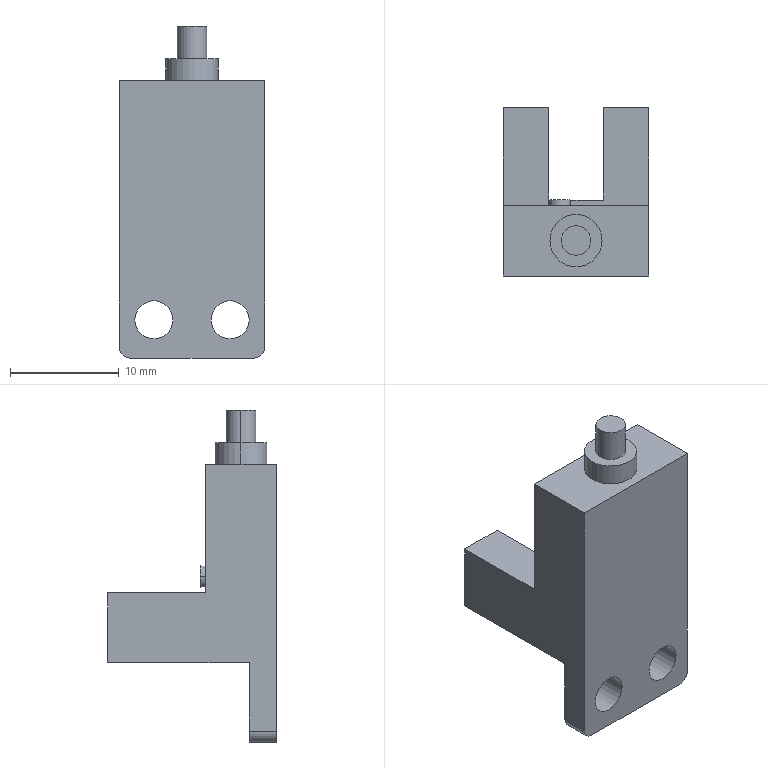Part | STEP file | PM-Y44 | 1 solid | 160 faces | box 13.4 x 15.5 x 30.5 mm | volume 2335 mm3 | plane 120 | spline 28 | cylinder 12 | commonest cylinder face diameters 2 x4 3.5 x4 2.7 x2 4.8 x2